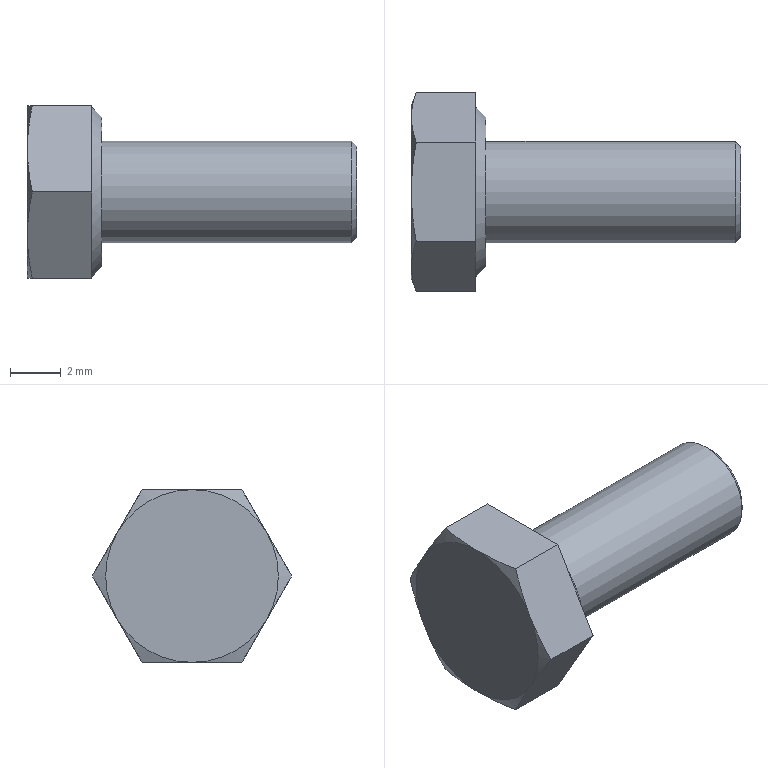Part | STEP file | hexagon head bolts-full thread gb_GB_FASTENER_BOLT_STBAB A M4X10-N | 1 solid | 19 faces | box 12.925 x 7.829 x 6.78 mm | volume 238.129 mm3 | plane 10 | cone 8 | cylinder 1 | commonest cylinder face diameters 4 x1